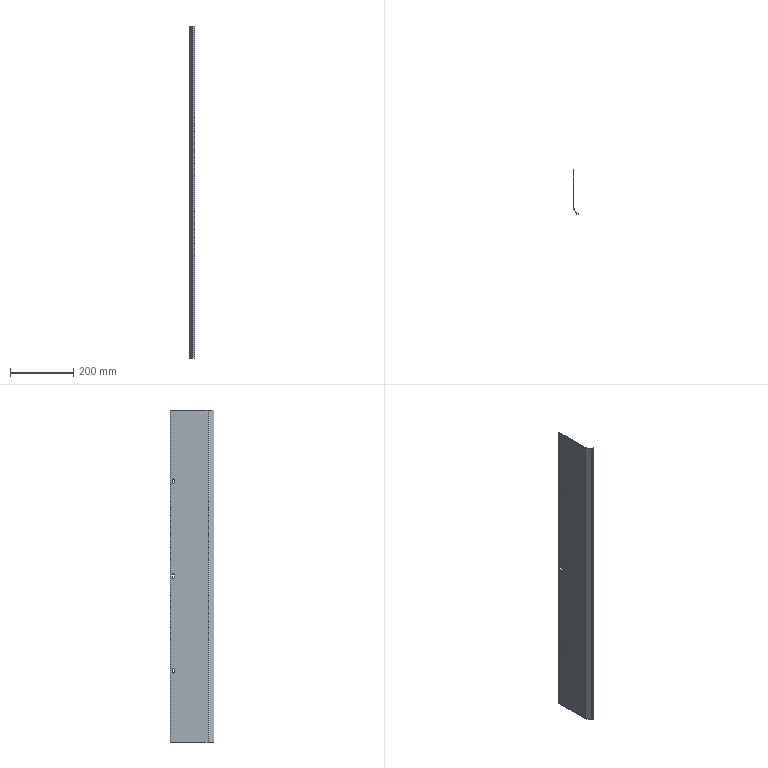Part | SolidWorks | features FlatPattern 1, ICE 1, SMBaseFlange 1, SheetMetal 1 | 1 solid | 37 faces | box 17 x 138.321 x 1050 mm | volume 153799 mm3 | plane 24 | cylinder 13 | commonest cylinder face diameters 7 x9 1 x2 3 x2
STEP:
#1=CARTESIAN_POINT('',(0.,-6.5,-296.5));
#2=VERTEX_POINT('',#1);
#3=CARTESIAN_POINT('',(0.,-10.,-293.));
#4=VERTEX_POINT('',#3);
#5=CARTESIAN_POINT('',(0.,-10.,-296.5));
#6=DIRECTION('',(1.,0.,0.));
#7=DIRECTION('',(0.,1.,0.));
#8=AXIS2_PLACEMENT_3D('',#5,#6,#7);
#9=CIRCLE('',#8,3.5);
#10=EDGE_CURVE('',#2,#4,#9,.T.);
#11=ORIENTED_EDGE('',*,*,#10,.T.);
#12=CARTESIAN_POINT('',(-1.,-10.,-293.));
#13=VERTEX_POINT('',#12);
#14=CARTESIAN_POINT('',(9.,-10.,-293.));
#15=DIRECTION('',(-1.,0.,0.));
#16=VECTOR('',#15,1000.);
#17=LINE('',#14,#16);
#18=EDGE_CURVE('',#4,#13,#17,.T.);
#19=ORIENTED_EDGE('',*,*,#18,.T.);
#20=CARTESIAN_POINT('',(-1.,-6.5,-296.5));
#21=VERTEX_POINT('',#20);
#22=CARTESIAN_POINT('',(-1.,-10.,-296.5));
#23=DIRECTION('',(-1.,0.,0.));
#24=DIRECTION('',(0.,0.,1.));
#25=AXIS2_PLACEMENT_3D('',#22,#23,#24);
#26=CIRCLE('',#25,3.5);
#27=EDGE_CURVE('',#13,#21,#26,.T.);
#28=ORIENTED_EDGE('',*,*,#27,.T.);
#29=CARTESIAN_POINT('',(9.,-6.5,-296.5));
#30=DIRECTION('',(-1.,0.,0.));
#31=VECTOR('',#30,1000.);
#32=LINE('',#29,#31);
#33=EDGE_CURVE('',#2,#21,#32,.T.);
#34=ORIENTED_EDGE('',*,*,#33,.F.);
#35=EDGE_LOOP('',(#11,#19,#28,#34));
#36=FACE_OUTER_BOUND('',#35,.T.);
#37=CARTESIAN_POINT('',(9.,-10.,-296.5));
#38=DIRECTION('',(-1.,0.,0.));
#39=DIRECTION('',(0.,0.,1.));
#40=AXIS2_PLACEMENT_3D('',#37,#38,#39);
#41=CYLINDRICAL_SURFACE('',#40,3.5);
#42=ADVANCED_FACE('',(#36),#41,.F.);
#43=CARTESIAN_POINT('',(0.,-6.5,303.5));
#44=VERTEX_POINT('',#43);
#45=CARTESIAN_POINT('',(0.,-10.,307.));
#46=VERTEX_POINT('',#45);
#47=CARTESIAN_POINT('',(0.,-10.,303.5));
#48=DIRECTION('',(1.,0.,0.));
#49=DIRECTION('',(0.,1.,0.));
#50=AXIS2_PLACEMENT_3D('',#47,#48,#49);
#51=CIRCLE('',#50,3.5);
#52=EDGE_CURVE('',#44,#46,#51,.T.);
#53=ORIENTED_EDGE('',*,*,#52,.T.);
#54=CARTESIAN_POINT('',(-1.,-10.,307.));
#55=VERTEX_POINT('',#54);
#56=CARTESIAN_POINT('',(9.,-10.,307.));
#57=DIRECTION('',(-1.,0.,0.));
#58=VECTOR('',#57,1000.);
#59=LINE('',#56,#58);
#60=EDGE_CURVE('',#46,#55,#59,.T.);
#61=ORIENTED_EDGE('',*,*,#60,.T.);
#62=CARTESIAN_POINT('',(-1.,-6.5,303.5));
#63=VERTEX_POINT('',#62);
#64=CARTESIAN_POINT('',(-1.,-10.,303.5));
#65=DIRECTION('',(-1.,0.,0.));
#66=DIRECTION('',(0.,0.,1.));
#67=AXIS2_PLACEMENT_3D('',#64,#65,#66);
#68=CIRCLE('',#67,3.5);
#69=EDGE_CURVE('',#55,#63,#68,.T.);
#70=ORIENTED_EDGE('',*,*,#69,.T.);
#71=CARTESIAN_POINT('',(9.,-6.5,303.5));
#72=DIRECTION('',(-1.,0.,0.));
#73=VECTOR('',#72,1000.);
#74=LINE('',#71,#73);
#75=EDGE_CURVE('',#44,#63,#74,.T.);
#76=ORIENTED_EDGE('',*,*,#75,.F.);
#77=EDGE_LOOP('',(#53,#61,#70,#76));
#78=FACE_OUTER_BOUND('',#77,.T.);
#79=CARTESIAN_POINT('',(9.,-10.,303.5));
#80=DIRECTION('',(-1.,0.,0.));
#81=DIRECTION('',(0.,0.,1.));
#82=AXIS2_PLACEMENT_3D('',#79,#80,#81);
#83=CYLINDRICAL_SURFACE('',#82,3.5);
#84=ADVANCED_FACE('',(#78),#83,.F.);
#85=CARTESIAN_POINT('',(0.,-6.5,3.5));
#86=VERTEX_POINT('',#85);
#87=CARTESIAN_POINT('',(0.,-10.,7.));
#88=VERTEX_POINT('',#87);
#89=CARTESIAN_POINT('',(0.,-10.,3.5));
#90=DIRECTION('',(1.,0.,0.));
#91=DIRECTION('',(0.,1.,0.));
#92=AXIS2_PLACEMENT_3D('',#89,#90,#91);
#93=CIRCLE('',#92,3.5);
#94=EDGE_CURVE('',#86,#88,#93,.T.);
#95=ORIENTED_EDGE('',*,*,#94,.T.);
#96=CARTESIAN_POINT('',(-1.,-10.,7.));
#97=VERTEX_POINT('',#96);
#98=CARTESIAN_POINT('',(9.,-10.,7.));
#99=DIRECTION('',(-1.,0.,0.));
#100=VECTOR('',#99,1000.);
#101=LINE('',#98,#100);
#102=EDGE_CURVE('',#88,#97,#101,.T.);
#103=ORIENTED_EDGE('',*,*,#102,.T.);
#104=CARTESIAN_POINT('',(-1.,-6.5,3.5));
#105=VERTEX_POINT('',#104);
#106=CARTESIAN_POINT('',(-1.,-10.,3.5));
#107=DIRECTION('',(-1.,0.,0.));
#108=DIRECTION('',(0.,0.,1.));
#109=AXIS2_PLACEMENT_3D('',#106,#107,#108);
#110=CIRCLE('',#109,3.5);
#111=EDGE_CURVE('',#97,#105,#110,.T.);
#112=ORIENTED_EDGE('',*,*,#111,.T.);
#113=CARTESIAN_POINT('',(9.,-6.5,3.5));
#114=DIRECTION('',(-1.,0.,0.));
#115=VECTOR('',#114,1000.);
#116=LINE('',#113,#115);
#117=EDGE_CURVE('',#86,#105,#116,.T.);
#118=ORIENTED_EDGE('',*,*,#117,.F.);
#119=EDGE_LOOP('',(#95,#103,#112,#118));
#120=FACE_OUTER_BOUND('',#119,.T.);
#121=CARTESIAN_POINT('',(9.,-10.,3.5));
#122=DIRECTION('',(-1.,0.,0.));
#123=DIRECTION('',(0.,0.,1.));
#124=AXIS2_PLACEMENT_3D('',#121,#122,#123);
#125=CYLINDRICAL_SURFACE('',#124,3.5);
#126=ADVANCED_FACE('',(#120),#125,.F.);
#127=CARTESIAN_POINT('',(0.06699,-120.116,525.));
#128=VERTEX_POINT('',#127);
#129=CARTESIAN_POINT('',(-0.799,-120.616,525.));
#130=VERTEX_POINT('',#129);
#131=CARTESIAN_POINT('',(0.06699,-120.116,525.));
#132=DIRECTION('',(-0.866,-0.5,0.));
#133=VECTOR('',#132,1000.);
#134=LINE('',#131,#133);
#135=EDGE_CURVE('',#128,#130,#134,.T.);
#136=ORIENTED_EDGE('',*,*,#135,.F.);
#137=CARTESIAN_POINT('',(0.,-119.866,525.));
#138=VERTEX_POINT('',#137);
#139=CARTESIAN_POINT('',(0.5,-119.866,525.));
#140=DIRECTION('',(0.,0.,1.));
#141=DIRECTION('',(-1.,0.,0.));
#142=AXIS2_PLACEMENT_3D('',#139,#140,#141);
#143=CIRCLE('',#142,0.5);
#144=EDGE_CURVE('',#138,#128,#143,.T.);
#145=ORIENTED_EDGE('',*,*,#144,.F.);
#146=CARTESIAN_POINT('',(-1.,-119.866,525.));
#147=VERTEX_POINT('',#146);
#148=CARTESIAN_POINT('',(-1.,-119.866,525.));
#149=DIRECTION('',(1.,0.,0.));
#150=VECTOR('',#149,1000.);
#151=LINE('',#148,#150);
#152=EDGE_CURVE('',#147,#138,#151,.T.);
#153=ORIENTED_EDGE('',*,*,#152,.F.);
#154=CARTESIAN_POINT('',(0.5,-119.866,525.));
#155=DIRECTION('',(0.,0.,1.));
#156=DIRECTION('',(1.,0.,0.));
#157=AXIS2_PLACEMENT_3D('',#154,#155,#156);
#158=CIRCLE('',#157,1.5);
#159=EDGE_CURVE('',#147,#130,#158,.T.);
#160=ORIENTED_EDGE('',*,*,#159,.T.);
#161=EDGE_LOOP('',(#136,#145,#153,#160));
#162=FACE_OUTER_BOUND('',#161,.T.);
#163=CARTESIAN_POINT('',(0.06699,-120.116,525.));
#164=DIRECTION('',(0.,0.,1.));
#165=DIRECTION('',(1.,0.,0.));
#166=AXIS2_PLACEMENT_3D('',#163,#164,#165);
#167=PLANE('',#166);
#168=ADVANCED_FACE('',(#162),#167,.T.);
#169=CARTESIAN_POINT('',(9.856,-137.071,525.));
#170=VERTEX_POINT('',#169);
#171=CARTESIAN_POINT('',(0.,-120.,525.));
#172=DIRECTION('',(0.5,-0.866,0.));
#173=VECTOR('',#172,1000.);
#174=LINE('',#171,#173);
#175=EDGE_CURVE('',#128,#170,#174,.T.);
#176=ORIENTED_EDGE('',*,*,#175,.F.);
#177=ORIENTED_EDGE('',*,*,#135,.T.);
#178=CARTESIAN_POINT('',(8.99,-137.571,525.));
#179=VERTEX_POINT('',#178);
#180=CARTESIAN_POINT('',(-0.866,-120.5,525.));
#181=DIRECTION('',(0.5,-0.866,0.));
#182=VECTOR('',#181,1000.);
#183=LINE('',#180,#182);
#184=EDGE_CURVE('',#130,#179,#183,.T.);
#185=ORIENTED_EDGE('',*,*,#184,.T.);
#186=CARTESIAN_POINT('',(8.99,-137.571,525.));
#187=DIRECTION('',(0.866,0.5,0.));
#188=VECTOR('',#187,1000.);
#189=LINE('',#186,#188);
#190=EDGE_CURVE('',#179,#170,#189,.T.);
#191=ORIENTED_EDGE('',*,*,#190,.T.);
#192=EDGE_LOOP('',(#176,#177,#185,#191));
#193=FACE_OUTER_BOUND('',#192,.T.);
#194=CARTESIAN_POINT('',(-1.,-119.866,525.));
#195=DIRECTION('',(0.,0.,1.));
#196=DIRECTION('',(1.,0.,0.));
#197=AXIS2_PLACEMENT_3D('',#194,#195,#196);
#198=PLANE('',#197);
#199=ADVANCED_FACE('',(#193),#198,.T.);
#200=CARTESIAN_POINT('',(0.,-119.866,-525.));
#201=VERTEX_POINT('',#200);
#202=CARTESIAN_POINT('',(-1.,-119.866,-525.));
#203=VERTEX_POINT('',#202);
#204=CARTESIAN_POINT('',(0.,-119.866,-525.));
#205=DIRECTION('',(-1.,0.,0.));
#206=VECTOR('',#205,1000.);
#207=LINE('',#204,#206);
#208=EDGE_CURVE('',#201,#203,#207,.T.);
#209=ORIENTED_EDGE('',*,*,#208,.F.);
#210=CARTESIAN_POINT('',(0.06699,-120.116,-525.));
#211=VERTEX_POINT('',#210);
#212=CARTESIAN_POINT('',(0.5,-119.866,-525.));
#213=DIRECTION('',(0.,0.,1.));
#214=DIRECTION('',(-1.,0.,0.));
#215=AXIS2_PLACEMENT_3D('',#212,#213,#214);
#216=CIRCLE('',#215,0.5);
#217=EDGE_CURVE('',#201,#211,#216,.T.);
#218=ORIENTED_EDGE('',*,*,#217,.T.);
#219=CARTESIAN_POINT('',(-0.799,-120.616,-525.));
#220=VERTEX_POINT('',#219);
#221=CARTESIAN_POINT('',(-0.799,-120.616,-525.));
#222=DIRECTION('',(0.866,0.5,0.));
#223=VECTOR('',#222,1000.);
#224=LINE('',#221,#223);
#225=EDGE_CURVE('',#220,#211,#224,.T.);
#226=ORIENTED_EDGE('',*,*,#225,.F.);
#227=CARTESIAN_POINT('',(0.5,-119.866,-525.));
#228=DIRECTION('',(0.,0.,1.));
#229=DIRECTION('',(1.,0.,0.));
#230=AXIS2_PLACEMENT_3D('',#227,#228,#229);
#231=CIRCLE('',#230,1.5);
#232=EDGE_CURVE('',#203,#220,#231,.T.);
#233=ORIENTED_EDGE('',*,*,#232,.F.);
#234=EDGE_LOOP('',(#209,#218,#226,#233));
#235=FACE_OUTER_BOUND('',#234,.T.);
#236=CARTESIAN_POINT('',(0.,-119.866,-525.));
#237=DIRECTION('',(0.,0.,-1.));
#238=DIRECTION('',(-1.,0.,0.));
#239=AXIS2_PLACEMENT_3D('',#236,#237,#238);
#240=PLANE('',#239);
#241=ADVANCED_FACE('',(#235),#240,.T.);
#242=CARTESIAN_POINT('',(0.,0.,-525.));
#243=VERTEX_POINT('',#242);
#244=CARTESIAN_POINT('',(0.,0.,-525.));
#245=DIRECTION('',(0.,-1.,0.));
#246=VECTOR('',#245,1000.);
#247=LINE('',#244,#246);
#248=EDGE_CURVE('',#243,#201,#247,.T.);
#249=ORIENTED_EDGE('',*,*,#248,.T.);
#250=ORIENTED_EDGE('',*,*,#208,.T.);
#251=CARTESIAN_POINT('',(-1.,0.,-525.));
#252=VERTEX_POINT('',#251);
#253=CARTESIAN_POINT('',(-1.,0.,-525.));
#254=DIRECTION('',(0.,-1.,0.));
#255=VECTOR('',#254,1000.);
#256=LINE('',#253,#255);
#257=EDGE_CURVE('',#252,#203,#256,.T.);
#258=ORIENTED_EDGE('',*,*,#257,.F.);
#259=CARTESIAN_POINT('',(-1.,0.,-525.));
#260=DIRECTION('',(1.,0.,0.));
#261=VECTOR('',#260,1000.);
#262=LINE('',#259,#261);
#263=EDGE_CURVE('',#252,#243,#262,.T.);
#264=ORIENTED_EDGE('',*,*,#263,.T.);
#265=EDGE_LOOP('',(#249,#250,#258,#264));
#266=FACE_OUTER_BOUND('',#265,.T.);
#267=CARTESIAN_POINT('',(-0.799,-120.616,-525.));
#268=DIRECTION('',(0.,0.,-1.));
#269=DIRECTION('',(-1.,0.,0.));
#270=AXIS2_PLACEMENT_3D('',#267,#268,#269);
#271=PLANE('',#270);
#272=ADVANCED_FACE('',(#266),#271,.T.);
#273=CARTESIAN_POINT('',(10.289,-137.321,525.));
#274=VERTEX_POINT('',#273);
#275=CARTESIAN_POINT('',(10.289,-138.321,525.));
#276=VERTEX_POINT('',#275);
#277=CARTESIAN_POINT('',(10.289,-137.321,525.));
#278=DIRECTION('',(0.,-1.,0.));
#279=VECTOR('',#278,1000.);
#280=LINE('',#277,#279);
#281=EDGE_CURVE('',#274,#276,#280,.T.);
#282=ORIENTED_EDGE('',*,*,#281,.F.);
#283=CARTESIAN_POINT('',(10.289,-136.821,525.));
#284=DIRECTION('',(0.,0.,1.));
#285=DIRECTION('',(-1.,0.,0.));
#286=AXIS2_PLACEMENT_3D('',#283,#284,#285);
#287=CIRCLE('',#286,0.5);
#288=EDGE_CURVE('',#170,#274,#287,.T.);
#289=ORIENTED_EDGE('',*,*,#288,.F.);
#290=ORIENTED_EDGE('',*,*,#190,.F.);
#291=CARTESIAN_POINT('',(10.289,-136.821,525.));
#292=DIRECTION('',(0.,0.,1.));
#293=DIRECTION('',(1.,0.,0.));
#294=AXIS2_PLACEMENT_3D('',#291,#292,#293);
#295=CIRCLE('',#294,1.5);
#296=EDGE_CURVE('',#179,#276,#295,.T.);
#297=ORIENTED_EDGE('',*,*,#296,.T.);
#298=EDGE_LOOP('',(#282,#289,#290,#297));
#299=FACE_OUTER_BOUND('',#298,.T.);
#300=CARTESIAN_POINT('',(10.289,-137.321,525.));
#301=DIRECTION('',(0.,0.,1.));
#302=DIRECTION('',(1.,0.,0.));
#303=AXIS2_PLACEMENT_3D('',#300,#301,#302);
#304=PLANE('',#303);
#305=ADVANCED_FACE('',(#299),#304,.T.);
#306=CARTESIAN_POINT('',(16.,-137.321,525.));
#307=VERTEX_POINT('',#306);
#308=CARTESIAN_POINT('',(10.,-137.321,525.));
#309=DIRECTION('',(1.,0.,0.));
#310=VECTOR('',#309,1000.);
#311=LINE('',#308,#310);
#312=EDGE_CURVE('',#274,#307,#311,.T.);
#313=ORIENTED_EDGE('',*,*,#312,.F.);
#314=ORIENTED_EDGE('',*,*,#281,.T.);
#315=CARTESIAN_POINT('',(16.,-138.321,525.));
#316=VERTEX_POINT('',#315);
#317=CARTESIAN_POINT('',(10.,-138.321,525.));
#318=DIRECTION('',(1.,0.,0.));
#319=VECTOR('',#318,1000.);
#320=LINE('',#317,#319);
#321=EDGE_CURVE('',#276,#316,#320,.T.);
#322=ORIENTED_EDGE('',*,*,#321,.T.);
#323=CARTESIAN_POINT('',(16.,-137.321,525.));
#324=DIRECTION('',(0.,-1.,0.));
#325=VECTOR('',#324,1000.);
#326=LINE('',#323,#325);
#327=EDGE_CURVE('',#307,#316,#326,.T.);
#328=ORIENTED_EDGE('',*,*,#327,.F.);
#329=EDGE_LOOP('',(#313,#314,#322,#328));
#330=FACE_OUTER_BOUND('',#329,.T.);
#331=CARTESIAN_POINT('',(8.99,-137.571,525.));
#332=DIRECTION('',(0.,0.,1.));
#333=DIRECTION('',(1.,0.,0.));
#334=AXIS2_PLACEMENT_3D('',#331,#332,#333);
#335=PLANE('',#334);
#336=ADVANCED_FACE('',(#330),#335,.T.);
#337=CARTESIAN_POINT('',(9.856,-137.071,-525.));
#338=VERTEX_POINT('',#337);
#339=CARTESIAN_POINT('',(8.99,-137.571,-525.));
#340=VERTEX_POINT('',#339);
#341=CARTESIAN_POINT('',(9.856,-137.071,-525.));
#342=DIRECTION('',(-0.866,-0.5,0.));
#343=VECTOR('',#342,1000.);
#344=LINE('',#341,#343);
#345=EDGE_CURVE('',#338,#340,#344,.T.);
#346=ORIENTED_EDGE('',*,*,#345,.F.);
#347=CARTESIAN_POINT('',(10.289,-137.321,-525.));
#348=VERTEX_POINT('',#347);
#349=CARTESIAN_POINT('',(10.289,-136.821,-525.));
#350=DIRECTION('',(0.,0.,1.));
#351=DIRECTION('',(-1.,0.,0.));
#352=AXIS2_PLACEMENT_3D('',#349,#350,#351);
#353=CIRCLE('',#352,0.5);
#354=EDGE_CURVE('',#338,#348,#353,.T.);
#355=ORIENTED_EDGE('',*,*,#354,.T.);
#356=CARTESIAN_POINT('',(10.289,-138.321,-525.));
#357=VERTEX_POINT('',#356);
#358=CARTESIAN_POINT('',(10.289,-138.321,-525.));
#359=DIRECTION('',(0.,1.,0.));
#360=VECTOR('',#359,1000.);
#361=LINE('',#358,#360);
#362=EDGE_CURVE('',#357,#348,#361,.T.);
#363=ORIENTED_EDGE('',*,*,#362,.F.);
#364=CARTESIAN_POINT('',(10.289,-136.821,-525.));
#365=DIRECTION('',(0.,0.,1.));
#366=DIRECTION('',(1.,0.,0.));
#367=AXIS2_PLACEMENT_3D('',#364,#365,#366);
#368=CIRCLE('',#367,1.5);
#369=EDGE_CURVE('',#340,#357,#368,.T.);
#370=ORIENTED_EDGE('',*,*,#369,.F.);
#371=EDGE_LOOP('',(#346,#355,#363,#370));
#372=FACE_OUTER_BOUND('',#371,.T.);
#373=CARTESIAN_POINT('',(9.856,-137.071,-525.));
#374=DIRECTION('',(0.,0.,-1.));
#375=DIRECTION('',(-1.,0.,0.));
#376=AXIS2_PLACEMENT_3D('',#373,#374,#375);
#377=PLANE('',#376);
#378=ADVANCED_FACE('',(#372),#377,.T.);
#379=CARTESIAN_POINT('',(0.,-120.,-525.));
#380=DIRECTION('',(0.5,-0.866,0.));
#381=VECTOR('',#380,1000.);
#382=LINE('',#379,#381);
#383=EDGE_CURVE('',#211,#338,#382,.T.);
#384=ORIENTED_EDGE('',*,*,#383,.T.);
#385=ORIENTED_EDGE('',*,*,#345,.T.);
#386=CARTESIAN_POINT('',(-0.866,-120.5,-525.));
#387=DIRECTION('',(0.5,-0.866,0.));
#388=VECTOR('',#387,1000.);
#389=LINE('',#386,#388);
#390=EDGE_CURVE('',#220,#340,#389,.T.);
#391=ORIENTED_EDGE('',*,*,#390,.F.);
#392=ORIENTED_EDGE('',*,*,#225,.T.);
#393=EDGE_LOOP('',(#384,#385,#391,#392));
#394=FACE_OUTER_BOUND('',#393,.T.);
#395=CARTESIAN_POINT('',(10.289,-138.321,-525.));
#396=DIRECTION('',(0.,0.,-1.));
#397=DIRECTION('',(-1.,0.,0.));
#398=AXIS2_PLACEMENT_3D('',#395,#396,#397);
#399=PLANE('',#398);
#400=ADVANCED_FACE('',(#394),#399,.T.);
#401=CARTESIAN_POINT('',(16.,-138.321,-525.));
#402=VERTEX_POINT('',#401);
#403=CARTESIAN_POINT('',(10.,-138.321,-525.));
#404=DIRECTION('',(1.,0.,0.));
#405=VECTOR('',#404,1000.);
#406=LINE('',#403,#405);
#407=EDGE_CURVE('',#357,#402,#406,.T.);
#408=ORIENTED_EDGE('',*,*,#407,.T.);
#409=CARTESIAN_POINT('',(16.,-138.321,525.));
#410=DIRECTION('',(0.,0.,-1.));
#411=VECTOR('',#410,1000.);
#412=LINE('',#409,#411);
#413=EDGE_CURVE('',#316,#402,#412,.T.);
#414=ORIENTED_EDGE('',*,*,#413,.F.);
#415=ORIENTED_EDGE('',*,*,#321,.F.);
#416=CARTESIAN_POINT('',(10.289,-138.321,525.));
#417=DIRECTION('',(0.,0.,-1.));
#418=VECTOR('',#417,1000.);
#419=LINE('',#416,#418);
#420=EDGE_CURVE('',#276,#357,#419,.T.);
#421=ORIENTED_EDGE('',*,*,#420,.T.);
#422=EDGE_LOOP('',(#408,#414,#415,#421));
#423=FACE_OUTER_BOUND('',#422,.T.);
#424=CARTESIAN_POINT('',(10.,-138.321,525.));
#425=DIRECTION('',(0.,1.,0.));
#426=DIRECTION('',(0.,0.,1.));
#427=AXIS2_PLACEMENT_3D('',#424,#425,#426);
#428=PLANE('',#427);
#429=ADVANCED_FACE('',(#423),#428,.F.);
#430=CARTESIAN_POINT('',(16.,-137.321,-525.));
#431=VERTEX_POINT('',#430);
#432=CARTESIAN_POINT('',(16.,-137.321,-525.));
#433=DIRECTION('',(0.,-1.,0.));
#434=VECTOR('',#433,1000.);
#435=LINE('',#432,#434);
#436=EDGE_CURVE('',#431,#402,#435,.T.);
#437=ORIENTED_EDGE('',*,*,#436,.F.);
#438=CARTESIAN_POINT('',(16.,-137.321,525.));
#439=DIRECTION('',(0.,0.,-1.));
#440=VECTOR('',#439,1000.);
#441=LINE('',#438,#440);
#442=EDGE_CURVE('',#307,#431,#441,.T.);
#443=ORIENTED_EDGE('',*,*,#442,.F.);
#444=ORIENTED_EDGE('',*,*,#327,.T.);
#445=ORIENTED_EDGE('',*,*,#413,.T.);
#446=EDGE_LOOP('',(#437,#443,#444,#445));
#447=FACE_OUTER_BOUND('',#446,.T.);
#448=CARTESIAN_POINT('',(16.,-137.321,525.));
#449=DIRECTION('',(1.,0.,0.));
#450=DIRECTION('',(0.,0.,-1.));
#451=AXIS2_PLACEMENT_3D('',#448,#449,#450);
#452=PLANE('',#451);
#453=ADVANCED_FACE('',(#447),#452,.T.);
#454=CARTESIAN_POINT('',(10.,-137.321,-525.));
#455=DIRECTION('',(1.,0.,0.));
#456=VECTOR('',#455,1000.);
#457=LINE('',#454,#456);
#458=EDGE_CURVE('',#348,#431,#457,.T.);
#459=ORIENTED_EDGE('',*,*,#458,.F.);
#460=CARTESIAN_POINT('',(10.289,-137.321,525.));
#461=DIRECTION('',(0.,0.,-1.));
#462=VECTOR('',#461,1000.);
#463=LINE('',#460,#462);
#464=EDGE_CURVE('',#274,#348,#463,.T.);
#465=ORIENTED_EDGE('',*,*,#464,.F.);
#466=ORIENTED_EDGE('',*,*,#312,.T.);
#467=ORIENTED_EDGE('',*,*,#442,.T.);
#468=EDGE_LOOP('',(#459,#465,#466,#467));
#469=FACE_OUTER_BOUND('',#468,.T.);
#470=CARTESIAN_POINT('',(10.,-137.321,525.));
#471=DIRECTION('',(0.,1.,0.));
#472=DIRECTION('',(0.,0.,1.));
#473=AXIS2_PLACEMENT_3D('',#470,#471,#472);
#474=PLANE('',#473);
#475=ADVANCED_FACE('',(#469),#474,.T.);
#476=ORIENTED_EDGE('',*,*,#354,.F.);
#477=CARTESIAN_POINT('',(9.856,-137.071,525.));
#478=DIRECTION('',(0.,0.,-1.));
#479=VECTOR('',#478,1000.);
#480=LINE('',#477,#479);
#481=EDGE_CURVE('',#170,#338,#480,.T.);
#482=ORIENTED_EDGE('',*,*,#481,.F.);
#483=ORIENTED_EDGE('',*,*,#288,.T.);
#484=ORIENTED_EDGE('',*,*,#464,.T.);
#485=EDGE_LOOP('',(#476,#482,#483,#484));
#486=FACE_OUTER_BOUND('',#485,.T.);
#487=CARTESIAN_POINT('',(10.289,-136.821,525.));
#488=DIRECTION('',(0.,0.,-1.));
#489=DIRECTION('',(-1.,0.,0.));
#490=AXIS2_PLACEMENT_3D('',#487,#488,#489);
#491=CYLINDRICAL_SURFACE('',#490,0.5);
#492=ADVANCED_FACE('',(#486),#491,.F.);
#493=ORIENTED_EDGE('',*,*,#383,.F.);
#494=CARTESIAN_POINT('',(0.06699,-120.116,525.));
#495=DIRECTION('',(0.,0.,-1.));
#496=VECTOR('',#495,1000.);
#497=LINE('',#494,#496);
#498=EDGE_CURVE('',#128,#211,#497,.T.);
#499=ORIENTED_EDGE('',*,*,#498,.F.);
#500=ORIENTED_EDGE('',*,*,#175,.T.);
#501=ORIENTED_EDGE('',*,*,#481,.T.);
#502=EDGE_LOOP('',(#493,#499,#500,#501));
#503=FACE_OUTER_BOUND('',#502,.T.);
#504=CARTESIAN_POINT('',(0.,-120.,525.));
#505=DIRECTION('',(0.866,0.5,0.));
#506=DIRECTION('',(-0.5,0.866,0.));
#507=AXIS2_PLACEMENT_3D('',#504,#505,#506);
#508=PLANE('',#507);
#509=ADVANCED_FACE('',(#503),#508,.T.);
#510=ORIENTED_EDGE('',*,*,#217,.F.);
#511=CARTESIAN_POINT('',(0.,-119.866,525.));
#512=DIRECTION('',(0.,0.,-1.));
#513=VECTOR('',#512,1000.);
#514=LINE('',#511,#513);
#515=EDGE_CURVE('',#138,#201,#514,.T.);
#516=ORIENTED_EDGE('',*,*,#515,.F.);
#517=ORIENTED_EDGE('',*,*,#144,.T.);
#518=ORIENTED_EDGE('',*,*,#498,.T.);
#519=EDGE_LOOP('',(#510,#516,#517,#518));
#520=FACE_OUTER_BOUND('',#519,.T.);
#521=CARTESIAN_POINT('',(0.5,-119.866,525.));
#522=DIRECTION('',(0.,0.,-1.));
#523=DIRECTION('',(-1.,0.,0.));
#524=AXIS2_PLACEMENT_3D('',#521,#522,#523);
#525=CYLINDRICAL_SURFACE('',#524,0.5);
#526=ADVANCED_FACE('',(#520),#525,.F.);
#527=CARTESIAN_POINT('',(0.,-13.5,-303.5));
#528=VERTEX_POINT('',#527);
#529=CARTESIAN_POINT('',(0.,-6.5,-303.5));
#530=VERTEX_POINT('',#529);
#531=CARTESIAN_POINT('',(0.,-10.,-303.5));
#532=DIRECTION('',(1.,0.,0.));
#533=DIRECTION('',(0.,1.,0.));
#534=AXIS2_PLACEMENT_3D('',#531,#532,#533);
#535=CIRCLE('',#534,3.5);
#536=EDGE_CURVE('',#528,#530,#535,.T.);
#537=ORIENTED_EDGE('',*,*,#536,.F.);
#538=CARTESIAN_POINT('',(0.,-13.5,-296.5));
#539=VERTEX_POINT('',#538);
#540=CARTESIAN_POINT('',(0.,-13.5,525.));
#541=DIRECTION('',(0.,0.,-1.));
#542=VECTOR('',#541,1000.);
#543=LINE('',#540,#542);
#544=EDGE_CURVE('',#539,#528,#543,.T.);
#545=ORIENTED_EDGE('',*,*,#544,.F.);
#546=CARTESIAN_POINT('',(0.,-10.,-296.5));
#547=DIRECTION('',(1.,0.,0.));
#548=DIRECTION('',(0.,1.,0.));
#549=AXIS2_PLACEMENT_3D('',#546,#547,#548);
#550=CIRCLE('',#549,3.5);
#551=EDGE_CURVE('',#4,#539,#550,.T.);
#552=ORIENTED_EDGE('',*,*,#551,.F.);
#553=ORIENTED_EDGE('',*,*,#10,.F.);
#554=CARTESIAN_POINT('',(0.,-6.5,525.));
#555=DIRECTION('',(0.,0.,1.));
#556=VECTOR('',#555,1000.);
#557=LINE('',#554,#556);
#558=EDGE_CURVE('',#530,#2,#557,.T.);
#559=ORIENTED_EDGE('',*,*,#558,.F.);
#560=EDGE_LOOP('',(#537,#545,#552,#553,#559));
#561=FACE_BOUND('',#560,.T.);
#562=CARTESIAN_POINT('',(0.,-13.5,296.5));
#563=VERTEX_POINT('',#562);
#564=CARTESIAN_POINT('',(0.,-6.5,296.5));
#565=VERTEX_POINT('',#564);
#566=CARTESIAN_POINT('',(0.,-10.,296.5));
#567=DIRECTION('',(1.,0.,0.));
#568=DIRECTION('',(0.,1.,0.));
#569=AXIS2_PLACEMENT_3D('',#566,#567,#568);
#570=CIRCLE('',#569,3.5);
#571=EDGE_CURVE('',#563,#565,#570,.T.);
#572=ORIENTED_EDGE('',*,*,#571,.F.);
#573=CARTESIAN_POINT('',(0.,-13.5,303.5));
#574=VERTEX_POINT('',#573);
#575=CARTESIAN_POINT('',(0.,-13.5,525.));
#576=DIRECTION('',(0.,0.,-1.));
#577=VECTOR('',#576,1000.);
#578=LINE('',#575,#577);
#579=EDGE_CURVE('',#574,#563,#578,.T.);
#580=ORIENTED_EDGE('',*,*,#579,.F.);
#581=CARTESIAN_POINT('',(0.,-10.,303.5));
#582=DIRECTION('',(1.,0.,0.));
#583=DIRECTION('',(0.,1.,0.));
#584=AXIS2_PLACEMENT_3D('',#581,#582,#583);
#585=CIRCLE('',#584,3.5);
#586=EDGE_CURVE('',#46,#574,#585,.T.);
#587=ORIENTED_EDGE('',*,*,#586,.F.);
#588=ORIENTED_EDGE('',*,*,#52,.F.);
#589=CARTESIAN_POINT('',(0.,-6.5,525.));
#590=DIRECTION('',(0.,0.,1.));
#591=VECTOR('',#590,1000.);
#592=LINE('',#589,#591);
#593=EDGE_CURVE('',#565,#44,#592,.T.);
#594=ORIENTED_EDGE('',*,*,#593,.F.);
#595=EDGE_LOOP('',(#572,#580,#587,#588,#594));
#596=FACE_BOUND('',#595,.T.);
#597=CARTESIAN_POINT('',(0.,-13.5,-3.5));
#598=VERTEX_POINT('',#597);
#599=CARTESIAN_POINT('',(0.,-6.5,-3.5));
#600=VERTEX_POINT('',#599);
#601=CARTESIAN_POINT('',(0.,-10.,-3.5));
#602=DIRECTION('',(1.,0.,0.));
#603=DIRECTION('',(0.,1.,0.));
#604=AXIS2_PLACEMENT_3D('',#601,#602,#603);
#605=CIRCLE('',#604,3.5);
#606=EDGE_CURVE('',#598,#600,#605,.T.);
#607=ORIENTED_EDGE('',*,*,#606,.F.);
#608=CARTESIAN_POINT('',(0.,-13.5,3.5));
#609=VERTEX_POINT('',#608);
#610=CARTESIAN_POINT('',(0.,-13.5,525.));
#611=DIRECTION('',(0.,0.,-1.));
#612=VECTOR('',#611,1000.);
#613=LINE('',#610,#612);
#614=EDGE_CURVE('',#609,#598,#613,.T.);
#615=ORIENTED_EDGE('',*,*,#614,.F.);
#616=CARTESIAN_POINT('',(0.,-10.,3.5));
#617=DIRECTION('',(1.,0.,0.));
#618=DIRECTION('',(0.,1.,0.));
#619=AXIS2_PLACEMENT_3D('',#616,#617,#618);
#620=CIRCLE('',#619,3.5);
#621=EDGE_CURVE('',#88,#609,#620,.T.);
#622=ORIENTED_EDGE('',*,*,#621,.F.);
#623=ORIENTED_EDGE('',*,*,#94,.F.);
#624=CARTESIAN_POINT('',(0.,-6.5,525.));
#625=DIRECTION('',(0.,0.,1.));
#626=VECTOR('',#625,1000.);
#627=LINE('',#624,#626);
#628=EDGE_CURVE('',#600,#86,#627,.T.);
#629=ORIENTED_EDGE('',*,*,#628,.F.);
#630=EDGE_LOOP('',(#607,#615,#622,#623,#629));
#631=FACE_BOUND('',#630,.T.);
#632=ORIENTED_EDGE('',*,*,#248,.F.);
#633=CARTESIAN_POINT('',(0.,0.,525.));
#634=VERTEX_POINT('',#633);
#635=CARTESIAN_POINT('',(0.,0.,525.));
#636=DIRECTION('',(0.,0.,-1.));
#637=VECTOR('',#636,1000.);
#638=LINE('',#635,#637);
#639=EDGE_CURVE('',#634,#243,#638,.T.);
#640=ORIENTED_EDGE('',*,*,#639,.F.);
#641=CARTESIAN_POINT('',(0.,0.,525.));
#642=DIRECTION('',(0.,-1.,0.));
#643=VECTOR('',#642,1000.);
#644=LINE('',#641,#643);
#645=EDGE_CURVE('',#634,#138,#644,.T.);
#646=ORIENTED_EDGE('',*,*,#645,.T.);
#647=ORIENTED_EDGE('',*,*,#515,.T.);
#648=EDGE_LOOP('',(#632,#640,#646,#647));
#649=FACE_OUTER_BOUND('',#648,.T.);
#650=CARTESIAN_POINT('',(0.,0.,525.));
#651=DIRECTION('',(1.,0.,0.));
#652=DIRECTION('',(0.,1.,0.));
#653=AXIS2_PLACEMENT_3D('',#650,#651,#652);
#654=PLANE('',#653);
#655=ADVANCED_FACE('',(#561,#596,#631,#649),#654,.T.);
#656=ORIENTED_EDGE('',*,*,#263,.F.);
#657=CARTESIAN_POINT('',(-1.,0.,525.));
#658=VERTEX_POINT('',#657);
#659=CARTESIAN_POINT('',(-1.,0.,525.));
#660=DIRECTION('',(0.,0.,-1.));
#661=VECTOR('',#660,1000.);
#662=LINE('',#659,#661);
#663=EDGE_CURVE('',#658,#252,#662,.T.);
#664=ORIENTED_EDGE('',*,*,#663,.F.);
#665=CARTESIAN_POINT('',(-1.,0.,525.));
#666=DIRECTION('',(1.,0.,0.));
#667=VECTOR('',#666,1000.);
#668=LINE('',#665,#667);
#669=EDGE_CURVE('',#658,#634,#668,.T.);
#670=ORIENTED_EDGE('',*,*,#669,.T.);
#671=ORIENTED_EDGE('',*,*,#639,.T.);
#672=EDGE_LOOP('',(#656,#664,#670,#671));
#673=FACE_OUTER_BOUND('',#672,.T.);
#674=CARTESIAN_POINT('',(-1.,0.,525.));
#675=DIRECTION('',(0.,1.,0.));
#676=DIRECTION('',(-1.,0.,0.));
#677=AXIS2_PLACEMENT_3D('',#674,#675,#676);
#678=PLANE('',#677);
#679=ADVANCED_FACE('',(#673),#678,.T.);
#680=CARTESIAN_POINT('',(-1.,-13.5,-303.5));
#681=VERTEX_POINT('',#680);
#682=CARTESIAN_POINT('',(-1.,-13.5,-296.5));
#683=VERTEX_POINT('',#682);
#684=CARTESIAN_POINT('',(-1.,-13.5,-303.5));
#685=DIRECTION('',(0.,0.,1.));
#686=VECTOR('',#685,1000.);
#687=LINE('',#684,#686);
#688=EDGE_CURVE('',#681,#683,#687,.T.);
#689=ORIENTED_EDGE('',*,*,#688,.F.);
#690=CARTESIAN_POINT('',(-1.,-6.5,-303.5));
#691=VERTEX_POINT('',#690);
#692=CARTESIAN_POINT('',(-1.,-10.,-303.5));
#693=DIRECTION('',(-1.,0.,0.));
#694=DIRECTION('',(0.,0.,1.));
#695=AXIS2_PLACEMENT_3D('',#692,#693,#694);
#696=CIRCLE('',#695,3.5);
#697=EDGE_CURVE('',#691,#681,#696,.T.);
#698=ORIENTED_EDGE('',*,*,#697,.F.);
#699=CARTESIAN_POINT('',(-1.,-6.5,-303.5));
#700=DIRECTION('',(0.,0.,-1.));
#701=VECTOR('',#700,1000.);
#702=LINE('',#699,#701);
#703=EDGE_CURVE('',#21,#691,#702,.T.);
#704=ORIENTED_EDGE('',*,*,#703,.F.);
#705=ORIENTED_EDGE('',*,*,#27,.F.);
#706=CARTESIAN_POINT('',(-1.,-10.,-296.5));
#707=DIRECTION('',(-1.,0.,0.));
#708=DIRECTION('',(0.,0.,1.));
#709=AXIS2_PLACEMENT_3D('',#706,#707,#708);
#710=CIRCLE('',#709,3.5);
#711=EDGE_CURVE('',#683,#13,#710,.T.);
#712=ORIENTED_EDGE('',*,*,#711,.F.);
#713=EDGE_LOOP('',(#689,#698,#704,#705,#712));
#714=FACE_BOUND('',#713,.T.);
#715=CARTESIAN_POINT('',(-1.,-13.5,296.5));
#716=VERTEX_POINT('',#715);
#717=CARTESIAN_POINT('',(-1.,-13.5,303.5));
#718=VERTEX_POINT('',#717);
#719=CARTESIAN_POINT('',(-1.,-13.5,296.5));
#720=DIRECTION('',(0.,0.,1.));
#721=VECTOR('',#720,1000.);
#722=LINE('',#719,#721);
#723=EDGE_CURVE('',#716,#718,#722,.T.);
#724=ORIENTED_EDGE('',*,*,#723,.F.);
#725=CARTESIAN_POINT('',(-1.,-6.5,296.5));
#726=VERTEX_POINT('',#725);
#727=CARTESIAN_POINT('',(-1.,-10.,296.5));
#728=DIRECTION('',(-1.,0.,0.));
#729=DIRECTION('',(0.,0.,1.));
#730=AXIS2_PLACEMENT_3D('',#727,#728,#729);
#731=CIRCLE('',#730,3.5);
#732=EDGE_CURVE('',#726,#716,#731,.T.);
#733=ORIENTED_EDGE('',*,*,#732,.F.);
#734=CARTESIAN_POINT('',(-1.,-6.5,296.5));
#735=DIRECTION('',(0.,0.,-1.));
#736=VECTOR('',#735,1000.);
#737=LINE('',#734,#736);
#738=EDGE_CURVE('',#63,#726,#737,.T.);
#739=ORIENTED_EDGE('',*,*,#738,.F.);
#740=ORIENTED_EDGE('',*,*,#69,.F.);
#741=CARTESIAN_POINT('',(-1.,-10.,303.5));
#742=DIRECTION('',(-1.,0.,0.));
#743=DIRECTION('',(0.,0.,1.));
#744=AXIS2_PLACEMENT_3D('',#741,#742,#743);
#745=CIRCLE('',#744,3.5);
#746=EDGE_CURVE('',#718,#55,#745,.T.);
#747=ORIENTED_EDGE('',*,*,#746,.F.);
#748=EDGE_LOOP('',(#724,#733,#739,#740,#747));
#749=FACE_BOUND('',#748,.T.);
#750=CARTESIAN_POINT('',(-1.,-13.5,-3.5));
#751=VERTEX_POINT('',#750);
#752=CARTESIAN_POINT('',(-1.,-13.5,3.5));
#753=VERTEX_POINT('',#752);
#754=CARTESIAN_POINT('',(-1.,-13.5,-3.5));
#755=DIRECTION('',(0.,0.,1.));
#756=VECTOR('',#755,1000.);
#757=LINE('',#754,#756);
#758=EDGE_CURVE('',#751,#753,#757,.T.);
#759=ORIENTED_EDGE('',*,*,#758,.F.);
#760=CARTESIAN_POINT('',(-1.,-6.5,-3.5));
#761=VERTEX_POINT('',#760);
#762=CARTESIAN_POINT('',(-1.,-10.,-3.5));
#763=DIRECTION('',(-1.,0.,0.));
#764=DIRECTION('',(0.,0.,1.));
#765=AXIS2_PLACEMENT_3D('',#762,#763,#764);
#766=CIRCLE('',#765,3.5);
#767=EDGE_CURVE('',#761,#751,#766,.T.);
#768=ORIENTED_EDGE('',*,*,#767,.F.);
#769=CARTESIAN_POINT('',(-1.,-6.5,-3.5));
#770=DIRECTION('',(0.,0.,-1.));
#771=VECTOR('',#770,1000.);
#772=LINE('',#769,#771);
#773=EDGE_CURVE('',#105,#761,#772,.T.);
#774=ORIENTED_EDGE('',*,*,#773,.F.);
#775=ORIENTED_EDGE('',*,*,#111,.F.);
#776=CARTESIAN_POINT('',(-1.,-10.,3.5));
#777=DIRECTION('',(-1.,0.,0.));
#778=DIRECTION('',(0.,0.,1.));
#779=AXIS2_PLACEMENT_3D('',#776,#777,#778);
#780=CIRCLE('',#779,3.5);
#781=EDGE_CURVE('',#753,#97,#780,.T.);
#782=ORIENTED_EDGE('',*,*,#781,.F.);
#783=EDGE_LOOP('',(#759,#768,#774,#775,#782));
#784=FACE_BOUND('',#783,.T.);
#785=ORIENTED_EDGE('',*,*,#257,.T.);
#786=CARTESIAN_POINT('',(-1.,-119.866,525.));
#787=DIRECTION('',(0.,0.,-1.));
#788=VECTOR('',#787,1000.);
#789=LINE('',#786,#788);
#790=EDGE_CURVE('',#147,#203,#789,.T.);
#791=ORIENTED_EDGE('',*,*,#790,.F.);
#792=CARTESIAN_POINT('',(-1.,0.,525.));
#793=DIRECTION('',(0.,-1.,0.));
#794=VECTOR('',#793,1000.);
#795=LINE('',#792,#794);
#796=EDGE_CURVE('',#658,#147,#795,.T.);
#797=ORIENTED_EDGE('',*,*,#796,.F.);
#798=ORIENTED_EDGE('',*,*,#663,.T.);
#799=EDGE_LOOP('',(#785,#791,#797,#798));
#800=FACE_OUTER_BOUND('',#799,.T.);
#801=CARTESIAN_POINT('',(-1.,0.,525.));
#802=DIRECTION('',(1.,0.,0.));
#803=DIRECTION('',(0.,1.,0.));
#804=AXIS2_PLACEMENT_3D('',#801,#802,#803);
#805=PLANE('',#804);
#806=ADVANCED_FACE('',(#714,#749,#784,#800),#805,.F.);
#807=ORIENTED_EDGE('',*,*,#232,.T.);
#808=CARTESIAN_POINT('',(-0.799,-120.616,525.));
#809=DIRECTION('',(0.,0.,-1.));
#810=VECTOR('',#809,1000.);
#811=LINE('',#808,#810);
#812=EDGE_CURVE('',#130,#220,#811,.T.);
#813=ORIENTED_EDGE('',*,*,#812,.F.);
#814=ORIENTED_EDGE('',*,*,#159,.F.);
#815=ORIENTED_EDGE('',*,*,#790,.T.);
#816=EDGE_LOOP('',(#807,#813,#814,#815));
#817=FACE_OUTER_BOUND('',#816,.T.);
#818=CARTESIAN_POINT('',(0.5,-119.866,525.));
#819=DIRECTION('',(0.,0.,-1.));
#820=DIRECTION('',(-1.,0.,0.));
#821=AXIS2_PLACEMENT_3D('',#818,#819,#820);
#822=CYLINDRICAL_SURFACE('',#821,1.5);
#823=ADVANCED_FACE('',(#817),#822,.T.);
#824=ORIENTED_EDGE('',*,*,#390,.T.);
#825=CARTESIAN_POINT('',(8.99,-137.571,525.));
#826=DIRECTION('',(0.,0.,-1.));
#827=VECTOR('',#826,1000.);
#828=LINE('',#825,#827);
#829=EDGE_CURVE('',#179,#340,#828,.T.);
#830=ORIENTED_EDGE('',*,*,#829,.F.);
#831=ORIENTED_EDGE('',*,*,#184,.F.);
#832=ORIENTED_EDGE('',*,*,#812,.T.);
#833=EDGE_LOOP('',(#824,#830,#831,#832));
#834=FACE_OUTER_BOUND('',#833,.T.);
#835=CARTESIAN_POINT('',(-0.866,-120.5,525.));
#836=DIRECTION('',(0.866,0.5,0.));
#837=DIRECTION('',(-0.5,0.866,0.));
#838=AXIS2_PLACEMENT_3D('',#835,#836,#837);
#839=PLANE('',#838);
#840=ADVANCED_FACE('',(#834),#839,.F.);
#841=ORIENTED_EDGE('',*,*,#369,.T.);
#842=ORIENTED_EDGE('',*,*,#420,.F.);
#843=ORIENTED_EDGE('',*,*,#296,.F.);
#844=ORIENTED_EDGE('',*,*,#829,.T.);
#845=EDGE_LOOP('',(#841,#842,#843,#844));
#846=FACE_OUTER_BOUND('',#845,.T.);
#847=CARTESIAN_POINT('',(10.289,-136.821,525.));
#848=DIRECTION('',(0.,0.,-1.));
#849=DIRECTION('',(-1.,0.,0.));
#850=AXIS2_PLACEMENT_3D('',#847,#848,#849);
#851=CYLINDRICAL_SURFACE('',#850,1.5);
#852=ADVANCED_FACE('',(#846),#851,.T.);
#853=ORIENTED_EDGE('',*,*,#796,.T.);
#854=ORIENTED_EDGE('',*,*,#152,.T.);
#855=ORIENTED_EDGE('',*,*,#645,.F.);
#856=ORIENTED_EDGE('',*,*,#669,.F.);
#857=EDGE_LOOP('',(#853,#854,#855,#856));
#858=FACE_OUTER_BOUND('',#857,.T.);
#859=CARTESIAN_POINT('',(10.289,-136.821,525.));
#860=DIRECTION('',(0.,0.,-1.));
#861=DIRECTION('',(-1.,0.,0.));
#862=AXIS2_PLACEMENT_3D('',#859,#860,#861);
#863=PLANE('',#862);
#864=ADVANCED_FACE('',(#858),#863,.F.);
#865=ORIENTED_EDGE('',*,*,#407,.F.);
#866=ORIENTED_EDGE('',*,*,#362,.T.);
#867=ORIENTED_EDGE('',*,*,#458,.T.);
#868=ORIENTED_EDGE('',*,*,#436,.T.);
#869=EDGE_LOOP('',(#865,#866,#867,#868));
#870=FACE_OUTER_BOUND('',#869,.T.);
#871=CARTESIAN_POINT('',(10.289,-136.821,-525.));
#872=DIRECTION('',(0.,0.,-1.));
#873=DIRECTION('',(-1.,0.,0.));
#874=AXIS2_PLACEMENT_3D('',#871,#872,#873);
#875=PLANE('',#874);
#876=ADVANCED_FACE('',(#870),#875,.T.);
#877=ORIENTED_EDGE('',*,*,#606,.T.);
#878=CARTESIAN_POINT('',(9.,-6.5,-3.5));
#879=DIRECTION('',(-1.,0.,0.));
#880=VECTOR('',#879,1000.);
#881=LINE('',#878,#880);
#882=EDGE_CURVE('',#600,#761,#881,.T.);
#883=ORIENTED_EDGE('',*,*,#882,.T.);
#884=ORIENTED_EDGE('',*,*,#767,.T.);
#885=CARTESIAN_POINT('',(9.,-13.5,-3.5));
#886=DIRECTION('',(-1.,0.,0.));
#887=VECTOR('',#886,1000.);
#888=LINE('',#885,#887);
#889=EDGE_CURVE('',#598,#751,#888,.T.);
#890=ORIENTED_EDGE('',*,*,#889,.F.);
#891=EDGE_LOOP('',(#877,#883,#884,#890));
#892=FACE_OUTER_BOUND('',#891,.T.);
#893=CARTESIAN_POINT('',(9.,-10.,-3.5));
#894=DIRECTION('',(-1.,0.,0.));
#895=DIRECTION('',(0.,0.,1.));
#896=AXIS2_PLACEMENT_3D('',#893,#894,#895);
#897=CYLINDRICAL_SURFACE('',#896,3.5);
#898=ADVANCED_FACE('',(#892),#897,.F.);
#899=ORIENTED_EDGE('',*,*,#628,.T.);
#900=ORIENTED_EDGE('',*,*,#117,.T.);
#901=ORIENTED_EDGE('',*,*,#773,.T.);
#902=ORIENTED_EDGE('',*,*,#882,.F.);
#903=EDGE_LOOP('',(#899,#900,#901,#902));
#904=FACE_OUTER_BOUND('',#903,.T.);
#905=CARTESIAN_POINT('',(9.,-6.5,-3.5));
#906=DIRECTION('',(0.,1.,0.));
#907=DIRECTION('',(0.,0.,1.));
#908=AXIS2_PLACEMENT_3D('',#905,#906,#907);
#909=PLANE('',#908);
#910=ADVANCED_FACE('',(#904),#909,.F.);
#911=ORIENTED_EDGE('',*,*,#102,.F.);
#912=ORIENTED_EDGE('',*,*,#621,.T.);
#913=CARTESIAN_POINT('',(9.,-13.5,3.5));
#914=DIRECTION('',(-1.,0.,0.));
#915=VECTOR('',#914,1000.);
#916=LINE('',#913,#915);
#917=EDGE_CURVE('',#609,#753,#916,.T.);
#918=ORIENTED_EDGE('',*,*,#917,.T.);
#919=ORIENTED_EDGE('',*,*,#781,.T.);
#920=EDGE_LOOP('',(#911,#912,#918,#919));
#921=FACE_OUTER_BOUND('',#920,.T.);
#922=CARTESIAN_POINT('',(9.,-10.,3.5));
#923=DIRECTION('',(-1.,0.,0.));
#924=DIRECTION('',(0.,0.,1.));
#925=AXIS2_PLACEMENT_3D('',#922,#923,#924);
#926=CYLINDRICAL_SURFACE('',#925,3.5);
#927=ADVANCED_FACE('',(#921),#926,.F.);
#928=ORIENTED_EDGE('',*,*,#614,.T.);
#929=ORIENTED_EDGE('',*,*,#889,.T.);
#930=ORIENTED_EDGE('',*,*,#758,.T.);
#931=ORIENTED_EDGE('',*,*,#917,.F.);
#932=EDGE_LOOP('',(#928,#929,#930,#931));
#933=FACE_OUTER_BOUND('',#932,.T.);
#934=CARTESIAN_POINT('',(9.,-13.5,-3.5));
#935=DIRECTION('',(0.,-1.,0.));
#936=DIRECTION('',(0.,0.,-1.));
#937=AXIS2_PLACEMENT_3D('',#934,#935,#936);
#938=PLANE('',#937);
#939=ADVANCED_FACE('',(#933),#938,.F.);
#940=ORIENTED_EDGE('',*,*,#571,.T.);
#941=CARTESIAN_POINT('',(9.,-6.5,296.5));
#942=DIRECTION('',(-1.,0.,0.));
#943=VECTOR('',#942,1000.);
#944=LINE('',#941,#943);
#945=EDGE_CURVE('',#565,#726,#944,.T.);
#946=ORIENTED_EDGE('',*,*,#945,.T.);
#947=ORIENTED_EDGE('',*,*,#732,.T.);
#948=CARTESIAN_POINT('',(9.,-13.5,296.5));
#949=DIRECTION('',(-1.,0.,0.));
#950=VECTOR('',#949,1000.);
#951=LINE('',#948,#950);
#952=EDGE_CURVE('',#563,#716,#951,.T.);
#953=ORIENTED_EDGE('',*,*,#952,.F.);
#954=EDGE_LOOP('',(#940,#946,#947,#953));
#955=FACE_OUTER_BOUND('',#954,.T.);
#956=CARTESIAN_POINT('',(9.,-10.,296.5));
#957=DIRECTION('',(-1.,0.,0.));
#958=DIRECTION('',(0.,0.,1.));
#959=AXIS2_PLACEMENT_3D('',#956,#957,#958);
#960=CYLINDRICAL_SURFACE('',#959,3.5);
#961=ADVANCED_FACE('',(#955),#960,.F.);
#962=ORIENTED_EDGE('',*,*,#593,.T.);
#963=ORIENTED_EDGE('',*,*,#75,.T.);
#964=ORIENTED_EDGE('',*,*,#738,.T.);
#965=ORIENTED_EDGE('',*,*,#945,.F.);
#966=EDGE_LOOP('',(#962,#963,#964,#965));
#967=FACE_OUTER_BOUND('',#966,.T.);
#968=CARTESIAN_POINT('',(9.,-6.5,296.5));
#969=DIRECTION('',(0.,1.,0.));
#970=DIRECTION('',(0.,0.,1.));
#971=AXIS2_PLACEMENT_3D('',#968,#969,#970);
#972=PLANE('',#971);
#973=ADVANCED_FACE('',(#967),#972,.F.);
#974=ORIENTED_EDGE('',*,*,#60,.F.);
#975=ORIENTED_EDGE('',*,*,#586,.T.);
#976=CARTESIAN_POINT('',(9.,-13.5,303.5));
#977=DIRECTION('',(-1.,0.,0.));
#978=VECTOR('',#977,1000.);
#979=LINE('',#976,#978);
#980=EDGE_CURVE('',#574,#718,#979,.T.);
#981=ORIENTED_EDGE('',*,*,#980,.T.);
#982=ORIENTED_EDGE('',*,*,#746,.T.);
#983=EDGE_LOOP('',(#974,#975,#981,#982));
#984=FACE_OUTER_BOUND('',#983,.T.);
#985=CARTESIAN_POINT('',(9.,-10.,303.5));
#986=DIRECTION('',(-1.,0.,0.));
#987=DIRECTION('',(0.,0.,1.));
#988=AXIS2_PLACEMENT_3D('',#985,#986,#987);
#989=CYLINDRICAL_SURFACE('',#988,3.5);
#990=ADVANCED_FACE('',(#984),#989,.F.);
#991=ORIENTED_EDGE('',*,*,#579,.T.);
#992=ORIENTED_EDGE('',*,*,#952,.T.);
#993=ORIENTED_EDGE('',*,*,#723,.T.);
#994=ORIENTED_EDGE('',*,*,#980,.F.);
#995=EDGE_LOOP('',(#991,#992,#993,#994));
#996=FACE_OUTER_BOUND('',#995,.T.);
#997=CARTESIAN_POINT('',(9.,-13.5,296.5));
#998=DIRECTION('',(0.,-1.,0.));
#999=DIRECTION('',(0.,0.,-1.));
#1000=AXIS2_PLACEMENT_3D('',#997,#998,#999);
#1001=PLANE('',#1000);
#1002=ADVANCED_FACE('',(#996),#1001,.F.);
#1003=ORIENTED_EDGE('',*,*,#536,.T.);
#1004=CARTESIAN_POINT('',(9.,-6.5,-303.5));
#1005=DIRECTION('',(-1.,0.,0.));
#1006=VECTOR('',#1005,1000.);
#1007=LINE('',#1004,#1006);
#1008=EDGE_CURVE('',#530,#691,#1007,.T.);
#1009=ORIENTED_EDGE('',*,*,#1008,.T.);
#1010=ORIENTED_EDGE('',*,*,#697,.T.);
#1011=CARTESIAN_POINT('',(9.,-13.5,-303.5));
#1012=DIRECTION('',(-1.,0.,0.));
#1013=VECTOR('',#1012,1000.);
#1014=LINE('',#1011,#1013);
#1015=EDGE_CURVE('',#528,#681,#1014,.T.);
#1016=ORIENTED_EDGE('',*,*,#1015,.F.);
#1017=EDGE_LOOP('',(#1003,#1009,#1010,#1016));
#1018=FACE_OUTER_BOUND('',#1017,.T.);
#1019=CARTESIAN_POINT('',(9.,-10.,-303.5));
#1020=DIRECTION('',(-1.,0.,0.));
#1021=DIRECTION('',(0.,0.,1.));
#1022=AXIS2_PLACEMENT_3D('',#1019,#1020,#1021);
#1023=CYLINDRICAL_SURFACE('',#1022,3.5);
#1024=ADVANCED_FACE('',(#1018),#1023,.F.);
#1025=ORIENTED_EDGE('',*,*,#558,.T.);
#1026=ORIENTED_EDGE('',*,*,#33,.T.);
#1027=ORIENTED_EDGE('',*,*,#703,.T.);
#1028=ORIENTED_EDGE('',*,*,#1008,.F.);
#1029=EDGE_LOOP('',(#1025,#1026,#1027,#1028));
#1030=FACE_OUTER_BOUND('',#1029,.T.);
#1031=CARTESIAN_POINT('',(9.,-6.5,-303.5));
#1032=DIRECTION('',(0.,1.,0.));
#1033=DIRECTION('',(0.,0.,1.));
#1034=AXIS2_PLACEMENT_3D('',#1031,#1032,#1033);
#1035=PLANE('',#1034);
#1036=ADVANCED_FACE('',(#1030),#1035,.F.);
#1037=ORIENTED_EDGE('',*,*,#18,.F.);
#1038=ORIENTED_EDGE('',*,*,#551,.T.);
#1039=CARTESIAN_POINT('',(9.,-13.5,-296.5));
#1040=DIRECTION('',(-1.,0.,0.));
#1041=VECTOR('',#1040,1000.);
#1042=LINE('',#1039,#1041);
#1043=EDGE_CURVE('',#539,#683,#1042,.T.);
#1044=ORIENTED_EDGE('',*,*,#1043,.T.);
#1045=ORIENTED_EDGE('',*,*,#711,.T.);
#1046=EDGE_LOOP('',(#1037,#1038,#1044,#1045));
#1047=FACE_OUTER_BOUND('',#1046,.T.);
#1048=CARTESIAN_POINT('',(9.,-10.,-296.5));
#1049=DIRECTION('',(-1.,0.,0.));
#1050=DIRECTION('',(0.,0.,1.));
#1051=AXIS2_PLACEMENT_3D('',#1048,#1049,#1050);
#1052=CYLINDRICAL_SURFACE('',#1051,3.5);
#1053=ADVANCED_FACE('',(#1047),#1052,.F.);
#1054=ORIENTED_EDGE('',*,*,#544,.T.);
#1055=ORIENTED_EDGE('',*,*,#1015,.T.);
#1056=ORIENTED_EDGE('',*,*,#688,.T.);
#1057=ORIENTED_EDGE('',*,*,#1043,.F.);
#1058=EDGE_LOOP('',(#1054,#1055,#1056,#1057));
#1059=FACE_OUTER_BOUND('',#1058,.T.);
#1060=CARTESIAN_POINT('',(9.,-13.5,-303.5));
#1061=DIRECTION('',(0.,-1.,0.));
#1062=DIRECTION('',(0.,0.,-1.));
#1063=AXIS2_PLACEMENT_3D('',#1060,#1061,#1062);
#1064=PLANE('',#1063);
#1065=ADVANCED_FACE('',(#1059),#1064,.F.);
#1066=CLOSED_SHELL('',(#42,#84,#126,#168,#199,#241,#272,#305,#336,#378,#400,#429,#453,#475,#492,#509,#526,#655,#679,#806,#823,#840,#852,#864,#876,#898,#910,#927,#939,#961,#973,#990,#1002,#1024,#1036,#1053,#1065));
#1067=MANIFOLD_SOLID_BREP('',#1066);
#1068=CARTESIAN_POINT('',(0.,0.,0.));
#1069=DIRECTION('',(0.,0.,1.));
#1070=DIRECTION('',(1.,0.,0.));
#1071=AXIS2_PLACEMENT_3D('',#1068,#1069,#1070);
#1072=(LENGTH_UNIT()NAMED_UNIT(*)SI_UNIT(.MILLI.,.METRE.));
#1073=UNCERTAINTY_MEASURE_WITH_UNIT(LENGTH_MEASURE(0.00001),#1072,'','');
#1074=(NAMED_UNIT(*)PLANE_ANGLE_UNIT()SI_UNIT($,.RADIAN.));
#1075=(NAMED_UNIT(*)SI_UNIT($,.STERADIAN.)SOLID_ANGLE_UNIT());
#1076=(GEOMETRIC_REPRESENTATION_CONTEXT(3)GLOBAL_UNCERTAINTY_ASSIGNED_CONTEXT((#1073))GLOBAL_UNIT_ASSIGNED_CONTEXT((#1072,#1074,#1075))REPRESENTATION_CONTEXT('',''));
#1077=ADVANCED_BREP_SHAPE_REPRESENTATION('',(#1067,#1071),#1076);